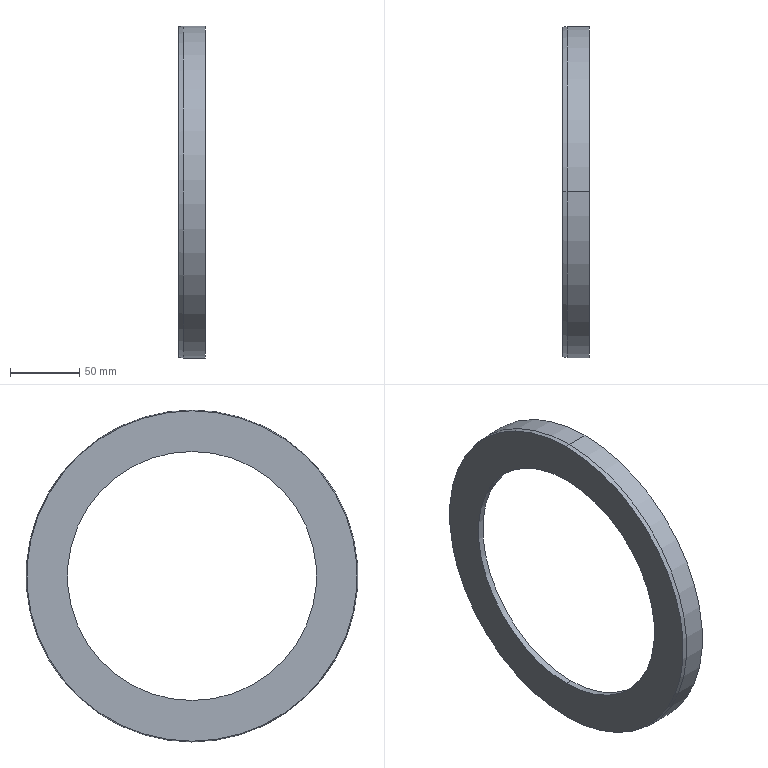Part | STEP file | Retaining ring | 1 solid | 13 faces | box 19 x 240 x 240 mm | volume 192307 mm3 | cylinder 6 | cone 4 | plane 3 | commonest cylinder face diameters 180 x2 220 x2 240 x2
STEP:
#1=CARTESIAN_POINT('',(0.,0.,0.));
#2=DIRECTION('',(0.,0.,1.));
#3=DIRECTION('',(1.,0.,0.));
#4=AXIS2_PLACEMENT_3D('',#1,#2,#3);
#5=CARTESIAN_POINT('',(4.5,0.,90.));
#6=VERTEX_POINT('',#5);
#7=CARTESIAN_POINT('',(0.,0.,90.));
#8=VERTEX_POINT('',#7);
#9=CARTESIAN_POINT('',(0.,0.,90.));
#10=DIRECTION('',(-1.,0.,0.));
#11=VECTOR('',#10,1.);
#12=LINE('',#9,#11);
#13=CARTESIAN_POINT('',(0.,0.,0.));
#14=DIRECTION('',(-1.,0.,0.));
#15=DIRECTION('',(0.,0.,1.));
#16=AXIS2_PLACEMENT_3D('',#13,#14,#15);
#17=CYLINDRICAL_SURFACE('',#16,90.);
#18=CARTESIAN_POINT('',(6.283,0.));
#19=DIRECTION('',(0.,1.));
#20=VECTOR('',#19,1.);
#21=LINE('',#18,#20);
#22=(GEOMETRIC_REPRESENTATION_CONTEXT(2)PARAMETRIC_REPRESENTATION_CONTEXT()REPRESENTATION_CONTEXT('',''));
#23=DEFINITIONAL_REPRESENTATION('',(#21),#22);
#24=PCURVE('',#17,#23);
#25=CARTESIAN_POINT('',(0.,0.,0.));
#26=DIRECTION('',(-1.,0.,0.));
#27=DIRECTION('',(0.,0.,1.));
#28=AXIS2_PLACEMENT_3D('',#25,#26,#27);
#29=CYLINDRICAL_SURFACE('',#28,90.);
#30=CARTESIAN_POINT('',(0.,0.));
#31=DIRECTION('',(0.,1.));
#32=VECTOR('',#31,1.);
#33=LINE('',#30,#32);
#34=(GEOMETRIC_REPRESENTATION_CONTEXT(2)PARAMETRIC_REPRESENTATION_CONTEXT()REPRESENTATION_CONTEXT('',''));
#35=DEFINITIONAL_REPRESENTATION('',(#33),#34);
#36=PCURVE('',#29,#35);
#37=SURFACE_CURVE('',#12,(#24,#36),.PCURVE_S1.);
#38=EDGE_CURVE('',#6,#8,#37,.T.);
#39=ORIENTED_EDGE('',*,*,#38,.T.);
#40=CARTESIAN_POINT('',(0.,0.,-90.));
#41=VERTEX_POINT('',#40);
#42=CARTESIAN_POINT('',(0.,0.,0.));
#43=DIRECTION('',(-1.,0.,0.));
#44=DIRECTION('',(0.,0.,1.));
#45=AXIS2_PLACEMENT_3D('',#42,#43,#44);
#46=CIRCLE('',#45,90.);
#47=CARTESIAN_POINT('',(0.,0.));
#48=DIRECTION('',(1.,0.));
#49=VECTOR('',#48,1.);
#50=LINE('',#47,#49);
#51=(GEOMETRIC_REPRESENTATION_CONTEXT(2)PARAMETRIC_REPRESENTATION_CONTEXT()REPRESENTATION_CONTEXT('',''));
#52=DEFINITIONAL_REPRESENTATION('',(#50),#51);
#53=PCURVE('',#17,#52);
#54=CARTESIAN_POINT('',(0.,-90.,0.));
#55=DIRECTION('',(-1.,0.,0.));
#56=DIRECTION('',(0.,0.,1.));
#57=AXIS2_PLACEMENT_3D('',#54,#55,#56);
#58=PLANE('',#57);
#59=CARTESIAN_POINT('',(0.,90.));
#60=DIRECTION('',(1.,0.));
#61=AXIS2_PLACEMENT_2D('',#59,#60);
#62=CIRCLE('',#61,90.);
#63=(GEOMETRIC_REPRESENTATION_CONTEXT(2)PARAMETRIC_REPRESENTATION_CONTEXT()REPRESENTATION_CONTEXT('',''));
#64=DEFINITIONAL_REPRESENTATION('',(#62),#63);
#65=PCURVE('',#58,#64);
#66=SURFACE_CURVE('',#46,(#53,#65),.PCURVE_S1.);
#67=EDGE_CURVE('',#41,#8,#66,.T.);
#68=ORIENTED_EDGE('',*,*,#67,.F.);
#69=CARTESIAN_POINT('',(4.5,0.,-90.));
#70=VERTEX_POINT('',#69);
#71=CARTESIAN_POINT('',(0.,0.,-90.));
#72=DIRECTION('',(-1.,0.,0.));
#73=VECTOR('',#72,1.);
#74=LINE('',#71,#73);
#75=CARTESIAN_POINT('',(3.142,0.));
#76=DIRECTION('',(0.,1.));
#77=VECTOR('',#76,1.);
#78=LINE('',#75,#77);
#79=(GEOMETRIC_REPRESENTATION_CONTEXT(2)PARAMETRIC_REPRESENTATION_CONTEXT()REPRESENTATION_CONTEXT('',''));
#80=DEFINITIONAL_REPRESENTATION('',(#78),#79);
#81=PCURVE('',#17,#80);
#82=CARTESIAN_POINT('',(3.142,0.));
#83=DIRECTION('',(0.,1.));
#84=VECTOR('',#83,1.);
#85=LINE('',#82,#84);
#86=(GEOMETRIC_REPRESENTATION_CONTEXT(2)PARAMETRIC_REPRESENTATION_CONTEXT()REPRESENTATION_CONTEXT('',''));
#87=DEFINITIONAL_REPRESENTATION('',(#85),#86);
#88=PCURVE('',#29,#87);
#89=SURFACE_CURVE('',#74,(#81,#88),.PCURVE_S1.);
#90=EDGE_CURVE('',#70,#41,#89,.T.);
#91=ORIENTED_EDGE('',*,*,#90,.F.);
#92=CARTESIAN_POINT('',(4.5,0.,0.));
#93=DIRECTION('',(-1.,0.,0.));
#94=DIRECTION('',(0.,0.,1.));
#95=AXIS2_PLACEMENT_3D('',#92,#93,#94);
#96=CIRCLE('',#95,90.);
#97=CARTESIAN_POINT('',(0.,-4.5));
#98=DIRECTION('',(1.,0.));
#99=VECTOR('',#98,1.);
#100=LINE('',#97,#99);
#101=(GEOMETRIC_REPRESENTATION_CONTEXT(2)PARAMETRIC_REPRESENTATION_CONTEXT()REPRESENTATION_CONTEXT('',''));
#102=DEFINITIONAL_REPRESENTATION('',(#100),#101);
#103=PCURVE('',#17,#102);
#104=CARTESIAN_POINT('',(4.5,-90.,0.));
#105=DIRECTION('',(1.,0.,0.));
#106=DIRECTION('',(0.,0.,-1.));
#107=AXIS2_PLACEMENT_3D('',#104,#105,#106);
#108=PLANE('',#107);
#109=CARTESIAN_POINT('',(-90.,90.));
#110=CARTESIAN_POINT('',(-90.,245.885));
#111=CARTESIAN_POINT('',(45.,167.942));
#112=CARTESIAN_POINT('',(180.,90.));
#113=CARTESIAN_POINT('',(45.,12.058));
#114=CARTESIAN_POINT('',(-90.,-65.885));
#115=CARTESIAN_POINT('',(-90.,90.));
#116=(BOUNDED_CURVE()B_SPLINE_CURVE(2,(#109,#110,#111,#112,#113,#114,#115),.UNSPECIFIED.,.T.,.F.)B_SPLINE_CURVE_WITH_KNOTS((1,2,2,2,2,1),(-2.094,0.,2.094,4.189,6.283,8.378),.UNSPECIFIED.)CURVE()GEOMETRIC_REPRESENTATION_ITEM()RATIONAL_B_SPLINE_CURVE((1.,0.5,1.,0.5,1.,0.5,1.))REPRESENTATION_ITEM(''));
#117=(GEOMETRIC_REPRESENTATION_CONTEXT(2)PARAMETRIC_REPRESENTATION_CONTEXT()REPRESENTATION_CONTEXT('',''));
#118=DEFINITIONAL_REPRESENTATION('',(#116),#117);
#119=PCURVE('',#108,#118);
#120=SURFACE_CURVE('',#96,(#103,#119),.PCURVE_S1.);
#121=EDGE_CURVE('',#70,#6,#120,.T.);
#122=ORIENTED_EDGE('',*,*,#121,.T.);
#123=EDGE_LOOP('',(#39,#68,#91,#122));
#124=FACE_BOUND('',#123,.F.);
#125=ADVANCED_FACE('',(#124),#17,.F.);
#126=CARTESIAN_POINT('',(0.,0.,119.408));
#127=VERTEX_POINT('',#126);
#128=CARTESIAN_POINT('',(0.,0.,-119.408));
#129=VERTEX_POINT('',#128);
#130=CARTESIAN_POINT('',(0.,0.,0.));
#131=DIRECTION('',(-1.,0.,0.));
#132=DIRECTION('',(0.,0.,1.));
#133=AXIS2_PLACEMENT_3D('',#130,#131,#132);
#134=CIRCLE('',#133,119.408);
#135=CARTESIAN_POINT('',(0.,0.,0.));
#136=DIRECTION('',(1.,0.,0.));
#137=DIRECTION('',(0.,0.,-1.));
#138=AXIS2_PLACEMENT_3D('',#135,#136,#137);
#139=CONICAL_SURFACE('',#138,119.408,0.1948);
#140=CARTESIAN_POINT('',(3.142,0.));
#141=DIRECTION('',(-1.,0.));
#142=VECTOR('',#141,1.);
#143=LINE('',#140,#142);
#144=(GEOMETRIC_REPRESENTATION_CONTEXT(2)PARAMETRIC_REPRESENTATION_CONTEXT()REPRESENTATION_CONTEXT('',''));
#145=DEFINITIONAL_REPRESENTATION('',(#143),#144);
#146=PCURVE('',#139,#145);
#147=CARTESIAN_POINT('',(0.,90.));
#148=DIRECTION('',(1.,0.));
#149=AXIS2_PLACEMENT_2D('',#147,#148);
#150=CIRCLE('',#149,119.408);
#151=(GEOMETRIC_REPRESENTATION_CONTEXT(2)PARAMETRIC_REPRESENTATION_CONTEXT()REPRESENTATION_CONTEXT('',''));
#152=DEFINITIONAL_REPRESENTATION('',(#150),#151);
#153=PCURVE('',#58,#152);
#154=SURFACE_CURVE('',#134,(#146,#153),.PCURVE_S1.);
#155=EDGE_CURVE('',#127,#129,#154,.T.);
#156=ORIENTED_EDGE('',*,*,#155,.F.);
#157=CARTESIAN_POINT('',(3.,0.,120.));
#158=VERTEX_POINT('',#157);
#159=CARTESIAN_POINT('',(0.,0.,119.408));
#160=DIRECTION('',(0.9811,0.,0.1936));
#161=VECTOR('',#160,1.);
#162=LINE('',#159,#161);
#163=CARTESIAN_POINT('',(3.142,0.));
#164=DIRECTION('',(0.,1.));
#165=VECTOR('',#164,1.);
#166=LINE('',#163,#165);
#167=(GEOMETRIC_REPRESENTATION_CONTEXT(2)PARAMETRIC_REPRESENTATION_CONTEXT()REPRESENTATION_CONTEXT('',''));
#168=DEFINITIONAL_REPRESENTATION('',(#166),#167);
#169=PCURVE('',#139,#168);
#170=CARTESIAN_POINT('',(0.,0.,0.));
#171=DIRECTION('',(1.,0.,0.));
#172=DIRECTION('',(0.,0.,-1.));
#173=AXIS2_PLACEMENT_3D('',#170,#171,#172);
#174=CONICAL_SURFACE('',#173,119.408,0.1948);
#175=CARTESIAN_POINT('',(3.142,0.));
#176=DIRECTION('',(0.,1.));
#177=VECTOR('',#176,1.);
#178=LINE('',#175,#177);
#179=(GEOMETRIC_REPRESENTATION_CONTEXT(2)PARAMETRIC_REPRESENTATION_CONTEXT()REPRESENTATION_CONTEXT('',''));
#180=DEFINITIONAL_REPRESENTATION('',(#178),#179);
#181=PCURVE('',#174,#180);
#182=SURFACE_CURVE('',#162,(#169,#181),.PCURVE_S1.);
#183=EDGE_CURVE('',#127,#158,#182,.T.);
#184=ORIENTED_EDGE('',*,*,#183,.T.);
#185=CARTESIAN_POINT('',(3.,0.,-120.));
#186=VERTEX_POINT('',#185);
#187=CARTESIAN_POINT('',(3.,0.,0.));
#188=DIRECTION('',(-1.,0.,0.));
#189=DIRECTION('',(0.,0.,1.));
#190=AXIS2_PLACEMENT_3D('',#187,#188,#189);
#191=CIRCLE('',#190,120.);
#192=CARTESIAN_POINT('',(3.142,3.));
#193=DIRECTION('',(-1.,0.));
#194=VECTOR('',#193,1.);
#195=LINE('',#192,#194);
#196=(GEOMETRIC_REPRESENTATION_CONTEXT(2)PARAMETRIC_REPRESENTATION_CONTEXT()REPRESENTATION_CONTEXT('',''));
#197=DEFINITIONAL_REPRESENTATION('',(#195),#196);
#198=PCURVE('',#139,#197);
#199=CARTESIAN_POINT('',(0.,0.,0.));
#200=DIRECTION('',(-1.,0.,0.));
#201=DIRECTION('',(0.,0.,1.));
#202=AXIS2_PLACEMENT_3D('',#199,#200,#201);
#203=CYLINDRICAL_SURFACE('',#202,120.);
#204=CARTESIAN_POINT('',(0.,-3.));
#205=DIRECTION('',(1.,0.));
#206=VECTOR('',#205,1.);
#207=LINE('',#204,#206);
#208=(GEOMETRIC_REPRESENTATION_CONTEXT(2)PARAMETRIC_REPRESENTATION_CONTEXT()REPRESENTATION_CONTEXT('',''));
#209=DEFINITIONAL_REPRESENTATION('',(#207),#208);
#210=PCURVE('',#203,#209);
#211=SURFACE_CURVE('',#191,(#198,#210),.PCURVE_S1.);
#212=EDGE_CURVE('',#158,#186,#211,.T.);
#213=ORIENTED_EDGE('',*,*,#212,.T.);
#214=CARTESIAN_POINT('',(0.,0.,-119.408));
#215=DIRECTION('',(0.9811,0.,-0.1936));
#216=VECTOR('',#215,1.);
#217=LINE('',#214,#216);
#218=CARTESIAN_POINT('',(0.,0.));
#219=DIRECTION('',(0.,1.));
#220=VECTOR('',#219,1.);
#221=LINE('',#218,#220);
#222=(GEOMETRIC_REPRESENTATION_CONTEXT(2)PARAMETRIC_REPRESENTATION_CONTEXT()REPRESENTATION_CONTEXT('',''));
#223=DEFINITIONAL_REPRESENTATION('',(#221),#222);
#224=PCURVE('',#139,#223);
#225=CARTESIAN_POINT('',(6.283,0.));
#226=DIRECTION('',(0.,1.));
#227=VECTOR('',#226,1.);
#228=LINE('',#225,#227);
#229=(GEOMETRIC_REPRESENTATION_CONTEXT(2)PARAMETRIC_REPRESENTATION_CONTEXT()REPRESENTATION_CONTEXT('',''));
#230=DEFINITIONAL_REPRESENTATION('',(#228),#229);
#231=PCURVE('',#174,#230);
#232=SURFACE_CURVE('',#217,(#224,#231),.PCURVE_S1.);
#233=EDGE_CURVE('',#129,#186,#232,.T.);
#234=ORIENTED_EDGE('',*,*,#233,.F.);
#235=EDGE_LOOP('',(#156,#184,#213,#234));
#236=FACE_BOUND('',#235,.T.);
#237=ADVANCED_FACE('',(#236),#139,.T.);
#238=CARTESIAN_POINT('',(19.,0.,120.));
#239=VERTEX_POINT('',#238);
#240=CARTESIAN_POINT('',(19.,0.,-120.));
#241=VERTEX_POINT('',#240);
#242=CARTESIAN_POINT('',(19.,0.,0.));
#243=DIRECTION('',(-1.,0.,0.));
#244=DIRECTION('',(0.,0.,1.));
#245=AXIS2_PLACEMENT_3D('',#242,#243,#244);
#246=CIRCLE('',#245,120.);
#247=CARTESIAN_POINT('',(0.,-19.));
#248=DIRECTION('',(1.,0.));
#249=VECTOR('',#248,1.);
#250=LINE('',#247,#249);
#251=(GEOMETRIC_REPRESENTATION_CONTEXT(2)PARAMETRIC_REPRESENTATION_CONTEXT()REPRESENTATION_CONTEXT('',''));
#252=DEFINITIONAL_REPRESENTATION('',(#250),#251);
#253=PCURVE('',#203,#252);
#254=CARTESIAN_POINT('',(19.,-112.473,0.));
#255=DIRECTION('',(1.,0.,0.));
#256=DIRECTION('',(0.,0.,-1.));
#257=AXIS2_PLACEMENT_3D('',#254,#255,#256);
#258=PLANE('',#257);
#259=CARTESIAN_POINT('',(-120.,112.473));
#260=CARTESIAN_POINT('',(-120.,320.32));
#261=CARTESIAN_POINT('',(60.,216.397));
#262=CARTESIAN_POINT('',(240.,112.473));
#263=CARTESIAN_POINT('',(60.,8.55));
#264=CARTESIAN_POINT('',(-120.,-95.373));
#265=CARTESIAN_POINT('',(-120.,112.473));
#266=(BOUNDED_CURVE()B_SPLINE_CURVE(2,(#259,#260,#261,#262,#263,#264,#265),.UNSPECIFIED.,.T.,.F.)B_SPLINE_CURVE_WITH_KNOTS((1,2,2,2,2,1),(-2.094,0.,2.094,4.189,6.283,8.378),.UNSPECIFIED.)CURVE()GEOMETRIC_REPRESENTATION_ITEM()RATIONAL_B_SPLINE_CURVE((1.,0.5,1.,0.5,1.,0.5,1.))REPRESENTATION_ITEM(''));
#267=(GEOMETRIC_REPRESENTATION_CONTEXT(2)PARAMETRIC_REPRESENTATION_CONTEXT()REPRESENTATION_CONTEXT('',''));
#268=DEFINITIONAL_REPRESENTATION('',(#266),#267);
#269=PCURVE('',#258,#268);
#270=SURFACE_CURVE('',#246,(#253,#269),.PCURVE_S1.);
#271=EDGE_CURVE('',#239,#241,#270,.T.);
#272=ORIENTED_EDGE('',*,*,#271,.T.);
#273=CARTESIAN_POINT('',(0.,0.,-120.));
#274=DIRECTION('',(-1.,0.,0.));
#275=VECTOR('',#274,1.);
#276=LINE('',#273,#275);
#277=CARTESIAN_POINT('',(3.142,0.));
#278=DIRECTION('',(0.,1.));
#279=VECTOR('',#278,1.);
#280=LINE('',#277,#279);
#281=(GEOMETRIC_REPRESENTATION_CONTEXT(2)PARAMETRIC_REPRESENTATION_CONTEXT()REPRESENTATION_CONTEXT('',''));
#282=DEFINITIONAL_REPRESENTATION('',(#280),#281);
#283=PCURVE('',#203,#282);
#284=CARTESIAN_POINT('',(0.,0.,0.));
#285=DIRECTION('',(-1.,0.,0.));
#286=DIRECTION('',(0.,0.,1.));
#287=AXIS2_PLACEMENT_3D('',#284,#285,#286);
#288=CYLINDRICAL_SURFACE('',#287,120.);
#289=CARTESIAN_POINT('',(3.142,0.));
#290=DIRECTION('',(0.,1.));
#291=VECTOR('',#290,1.);
#292=LINE('',#289,#291);
#293=(GEOMETRIC_REPRESENTATION_CONTEXT(2)PARAMETRIC_REPRESENTATION_CONTEXT()REPRESENTATION_CONTEXT('',''));
#294=DEFINITIONAL_REPRESENTATION('',(#292),#293);
#295=PCURVE('',#288,#294);
#296=SURFACE_CURVE('',#276,(#283,#295),.PCURVE_S1.);
#297=EDGE_CURVE('',#241,#186,#296,.T.);
#298=ORIENTED_EDGE('',*,*,#297,.T.);
#299=ORIENTED_EDGE('',*,*,#212,.F.);
#300=CARTESIAN_POINT('',(0.,0.,120.));
#301=DIRECTION('',(-1.,0.,0.));
#302=VECTOR('',#301,1.);
#303=LINE('',#300,#302);
#304=CARTESIAN_POINT('',(0.,0.));
#305=DIRECTION('',(0.,1.));
#306=VECTOR('',#305,1.);
#307=LINE('',#304,#306);
#308=(GEOMETRIC_REPRESENTATION_CONTEXT(2)PARAMETRIC_REPRESENTATION_CONTEXT()REPRESENTATION_CONTEXT('',''));
#309=DEFINITIONAL_REPRESENTATION('',(#307),#308);
#310=PCURVE('',#203,#309);
#311=CARTESIAN_POINT('',(6.283,0.));
#312=DIRECTION('',(0.,1.));
#313=VECTOR('',#312,1.);
#314=LINE('',#311,#313);
#315=(GEOMETRIC_REPRESENTATION_CONTEXT(2)PARAMETRIC_REPRESENTATION_CONTEXT()REPRESENTATION_CONTEXT('',''));
#316=DEFINITIONAL_REPRESENTATION('',(#314),#315);
#317=PCURVE('',#288,#316);
#318=SURFACE_CURVE('',#303,(#310,#317),.PCURVE_S1.);
#319=EDGE_CURVE('',#239,#158,#318,.T.);
#320=ORIENTED_EDGE('',*,*,#319,.F.);
#321=EDGE_LOOP('',(#272,#298,#299,#320));
#322=FACE_BOUND('',#321,.T.);
#323=ADVANCED_FACE('',(#322),#203,.T.);
#324=CARTESIAN_POINT('',(18.,0.,-110.));
#325=VERTEX_POINT('',#324);
#326=CARTESIAN_POINT('',(19.,0.,-112.473));
#327=VERTEX_POINT('',#326);
#328=CARTESIAN_POINT('',(19.,0.,-112.473));
#329=DIRECTION('',(0.3748,0.,-0.9271));
#330=VECTOR('',#329,1.);
#331=LINE('',#328,#330);
#332=CARTESIAN_POINT('',(19.,0.,0.));
#333=DIRECTION('',(1.,0.,0.));
#334=DIRECTION('',(0.,0.,-1.));
#335=AXIS2_PLACEMENT_3D('',#332,#333,#334);
#336=CONICAL_SURFACE('',#335,112.473,1.187);
#337=CARTESIAN_POINT('',(6.283,0.));
#338=DIRECTION('',(0.,1.));
#339=VECTOR('',#338,1.);
#340=LINE('',#337,#339);
#341=(GEOMETRIC_REPRESENTATION_CONTEXT(2)PARAMETRIC_REPRESENTATION_CONTEXT()REPRESENTATION_CONTEXT('',''));
#342=DEFINITIONAL_REPRESENTATION('',(#340),#341);
#343=PCURVE('',#336,#342);
#344=CARTESIAN_POINT('',(19.,0.,0.));
#345=DIRECTION('',(1.,0.,0.));
#346=DIRECTION('',(0.,0.,-1.));
#347=AXIS2_PLACEMENT_3D('',#344,#345,#346);
#348=CONICAL_SURFACE('',#347,112.473,1.187);
#349=CARTESIAN_POINT('',(0.,0.));
#350=DIRECTION('',(0.,1.));
#351=VECTOR('',#350,1.);
#352=LINE('',#349,#351);
#353=(GEOMETRIC_REPRESENTATION_CONTEXT(2)PARAMETRIC_REPRESENTATION_CONTEXT()REPRESENTATION_CONTEXT('',''));
#354=DEFINITIONAL_REPRESENTATION('',(#352),#353);
#355=PCURVE('',#348,#354);
#356=SURFACE_CURVE('',#331,(#343,#355),.PCURVE_S1.);
#357=EDGE_CURVE('',#325,#327,#356,.T.);
#358=ORIENTED_EDGE('',*,*,#357,.T.);
#359=CARTESIAN_POINT('',(19.,0.,112.473));
#360=VERTEX_POINT('',#359);
#361=CARTESIAN_POINT('',(19.,0.,0.));
#362=DIRECTION('',(-1.,0.,0.));
#363=DIRECTION('',(0.,0.,1.));
#364=AXIS2_PLACEMENT_3D('',#361,#362,#363);
#365=CIRCLE('',#364,112.473);
#366=CARTESIAN_POINT('',(9.425,0.));
#367=DIRECTION('',(-1.,0.));
#368=VECTOR('',#367,1.);
#369=LINE('',#366,#368);
#370=(GEOMETRIC_REPRESENTATION_CONTEXT(2)PARAMETRIC_REPRESENTATION_CONTEXT()REPRESENTATION_CONTEXT('',''));
#371=DEFINITIONAL_REPRESENTATION('',(#369),#370);
#372=PCURVE('',#336,#371);
#373=CARTESIAN_POINT('',(-112.473,112.473));
#374=CARTESIAN_POINT('',(-112.473,307.283));
#375=CARTESIAN_POINT('',(56.237,209.878));
#376=CARTESIAN_POINT('',(224.947,112.473));
#377=CARTESIAN_POINT('',(56.237,15.069));
#378=CARTESIAN_POINT('',(-112.473,-82.336));
#379=CARTESIAN_POINT('',(-112.473,112.473));
#380=(BOUNDED_CURVE()B_SPLINE_CURVE(2,(#373,#374,#375,#376,#377,#378,#379),.UNSPECIFIED.,.T.,.F.)B_SPLINE_CURVE_WITH_KNOTS((1,2,2,2,2,1),(-2.094,0.,2.094,4.189,6.283,8.378),.UNSPECIFIED.)CURVE()GEOMETRIC_REPRESENTATION_ITEM()RATIONAL_B_SPLINE_CURVE((1.,0.5,1.,0.5,1.,0.5,1.))REPRESENTATION_ITEM(''));
#381=(GEOMETRIC_REPRESENTATION_CONTEXT(2)PARAMETRIC_REPRESENTATION_CONTEXT()REPRESENTATION_CONTEXT('',''));
#382=DEFINITIONAL_REPRESENTATION('',(#380),#381);
#383=PCURVE('',#258,#382);
#384=SURFACE_CURVE('',#365,(#372,#383),.PCURVE_S1.);
#385=EDGE_CURVE('',#327,#360,#384,.T.);
#386=ORIENTED_EDGE('',*,*,#385,.T.);
#387=CARTESIAN_POINT('',(18.,0.,110.));
#388=VERTEX_POINT('',#387);
#389=CARTESIAN_POINT('',(19.,0.,112.473));
#390=DIRECTION('',(0.3748,0.,0.9271));
#391=VECTOR('',#390,1.);
#392=LINE('',#389,#391);
#393=CARTESIAN_POINT('',(3.142,0.));
#394=DIRECTION('',(0.,1.));
#395=VECTOR('',#394,1.);
#396=LINE('',#393,#395);
#397=(GEOMETRIC_REPRESENTATION_CONTEXT(2)PARAMETRIC_REPRESENTATION_CONTEXT()REPRESENTATION_CONTEXT('',''));
#398=DEFINITIONAL_REPRESENTATION('',(#396),#397);
#399=PCURVE('',#336,#398);
#400=CARTESIAN_POINT('',(3.142,0.));
#401=DIRECTION('',(0.,1.));
#402=VECTOR('',#401,1.);
#403=LINE('',#400,#402);
#404=(GEOMETRIC_REPRESENTATION_CONTEXT(2)PARAMETRIC_REPRESENTATION_CONTEXT()REPRESENTATION_CONTEXT('',''));
#405=DEFINITIONAL_REPRESENTATION('',(#403),#404);
#406=PCURVE('',#348,#405);
#407=SURFACE_CURVE('',#392,(#399,#406),.PCURVE_S1.);
#408=EDGE_CURVE('',#388,#360,#407,.T.);
#409=ORIENTED_EDGE('',*,*,#408,.F.);
#410=CARTESIAN_POINT('',(18.,0.,0.));
#411=DIRECTION('',(-1.,0.,0.));
#412=DIRECTION('',(0.,0.,1.));
#413=AXIS2_PLACEMENT_3D('',#410,#411,#412);
#414=CIRCLE('',#413,110.);
#415=CARTESIAN_POINT('',(9.425,-1.));
#416=DIRECTION('',(-1.,0.));
#417=VECTOR('',#416,1.);
#418=LINE('',#415,#417);
#419=(GEOMETRIC_REPRESENTATION_CONTEXT(2)PARAMETRIC_REPRESENTATION_CONTEXT()REPRESENTATION_CONTEXT('',''));
#420=DEFINITIONAL_REPRESENTATION('',(#418),#419);
#421=PCURVE('',#336,#420);
#422=CARTESIAN_POINT('',(0.,0.,0.));
#423=DIRECTION('',(-1.,0.,0.));
#424=DIRECTION('',(0.,0.,1.));
#425=AXIS2_PLACEMENT_3D('',#422,#423,#424);
#426=CYLINDRICAL_SURFACE('',#425,110.);
#427=CARTESIAN_POINT('',(0.,-18.));
#428=DIRECTION('',(1.,0.));
#429=VECTOR('',#428,1.);
#430=LINE('',#427,#429);
#431=(GEOMETRIC_REPRESENTATION_CONTEXT(2)PARAMETRIC_REPRESENTATION_CONTEXT()REPRESENTATION_CONTEXT('',''));
#432=DEFINITIONAL_REPRESENTATION('',(#430),#431);
#433=PCURVE('',#426,#432);
#434=SURFACE_CURVE('',#414,(#421,#433),.PCURVE_S1.);
#435=EDGE_CURVE('',#325,#388,#434,.T.);
#436=ORIENTED_EDGE('',*,*,#435,.F.);
#437=EDGE_LOOP('',(#358,#386,#409,#436));
#438=FACE_BOUND('',#437,.F.);
#439=ADVANCED_FACE('',(#438),#336,.F.);
#440=CARTESIAN_POINT('',(4.5,0.,110.));
#441=VERTEX_POINT('',#440);
#442=CARTESIAN_POINT('',(0.,0.,110.));
#443=DIRECTION('',(-1.,0.,0.));
#444=VECTOR('',#443,1.);
#445=LINE('',#442,#444);
#446=CARTESIAN_POINT('',(6.283,0.));
#447=DIRECTION('',(0.,1.));
#448=VECTOR('',#447,1.);
#449=LINE('',#446,#448);
#450=(GEOMETRIC_REPRESENTATION_CONTEXT(2)PARAMETRIC_REPRESENTATION_CONTEXT()REPRESENTATION_CONTEXT('',''));
#451=DEFINITIONAL_REPRESENTATION('',(#449),#450);
#452=PCURVE('',#426,#451);
#453=CARTESIAN_POINT('',(0.,0.,0.));
#454=DIRECTION('',(-1.,0.,0.));
#455=DIRECTION('',(0.,0.,1.));
#456=AXIS2_PLACEMENT_3D('',#453,#454,#455);
#457=CYLINDRICAL_SURFACE('',#456,110.);
#458=CARTESIAN_POINT('',(0.,0.));
#459=DIRECTION('',(0.,1.));
#460=VECTOR('',#459,1.);
#461=LINE('',#458,#460);
#462=(GEOMETRIC_REPRESENTATION_CONTEXT(2)PARAMETRIC_REPRESENTATION_CONTEXT()REPRESENTATION_CONTEXT('',''));
#463=DEFINITIONAL_REPRESENTATION('',(#461),#462);
#464=PCURVE('',#457,#463);
#465=SURFACE_CURVE('',#445,(#452,#464),.PCURVE_S1.);
#466=EDGE_CURVE('',#388,#441,#465,.T.);
#467=ORIENTED_EDGE('',*,*,#466,.T.);
#468=CARTESIAN_POINT('',(4.5,0.,-110.));
#469=VERTEX_POINT('',#468);
#470=CARTESIAN_POINT('',(4.5,0.,0.));
#471=DIRECTION('',(-1.,0.,0.));
#472=DIRECTION('',(0.,0.,1.));
#473=AXIS2_PLACEMENT_3D('',#470,#471,#472);
#474=CIRCLE('',#473,110.);
#475=CARTESIAN_POINT('',(0.,-4.5));
#476=DIRECTION('',(1.,0.));
#477=VECTOR('',#476,1.);
#478=LINE('',#475,#477);
#479=(GEOMETRIC_REPRESENTATION_CONTEXT(2)PARAMETRIC_REPRESENTATION_CONTEXT()REPRESENTATION_CONTEXT('',''));
#480=DEFINITIONAL_REPRESENTATION('',(#478),#479);
#481=PCURVE('',#426,#480);
#482=CARTESIAN_POINT('',(-110.,90.));
#483=CARTESIAN_POINT('',(-110.,280.526));
#484=CARTESIAN_POINT('',(55.,185.263));
#485=CARTESIAN_POINT('',(220.,90.));
#486=CARTESIAN_POINT('',(55.,-5.263));
#487=CARTESIAN_POINT('',(-110.,-100.526));
#488=CARTESIAN_POINT('',(-110.,90.));
#489=(BOUNDED_CURVE()B_SPLINE_CURVE(2,(#482,#483,#484,#485,#486,#487,#488),.UNSPECIFIED.,.T.,.F.)B_SPLINE_CURVE_WITH_KNOTS((1,2,2,2,2,1),(-2.094,0.,2.094,4.189,6.283,8.378),.UNSPECIFIED.)CURVE()GEOMETRIC_REPRESENTATION_ITEM()RATIONAL_B_SPLINE_CURVE((1.,0.5,1.,0.5,1.,0.5,1.))REPRESENTATION_ITEM(''));
#490=(GEOMETRIC_REPRESENTATION_CONTEXT(2)PARAMETRIC_REPRESENTATION_CONTEXT()REPRESENTATION_CONTEXT('',''));
#491=DEFINITIONAL_REPRESENTATION('',(#489),#490);
#492=PCURVE('',#108,#491);
#493=SURFACE_CURVE('',#474,(#481,#492),.PCURVE_S1.);
#494=EDGE_CURVE('',#469,#441,#493,.T.);
#495=ORIENTED_EDGE('',*,*,#494,.F.);
#496=CARTESIAN_POINT('',(0.,0.,-110.));
#497=DIRECTION('',(-1.,0.,0.));
#498=VECTOR('',#497,1.);
#499=LINE('',#496,#498);
#500=CARTESIAN_POINT('',(3.142,0.));
#501=DIRECTION('',(0.,1.));
#502=VECTOR('',#501,1.);
#503=LINE('',#500,#502);
#504=(GEOMETRIC_REPRESENTATION_CONTEXT(2)PARAMETRIC_REPRESENTATION_CONTEXT()REPRESENTATION_CONTEXT('',''));
#505=DEFINITIONAL_REPRESENTATION('',(#503),#504);
#506=PCURVE('',#426,#505);
#507=CARTESIAN_POINT('',(3.142,0.));
#508=DIRECTION('',(0.,1.));
#509=VECTOR('',#508,1.);
#510=LINE('',#507,#509);
#511=(GEOMETRIC_REPRESENTATION_CONTEXT(2)PARAMETRIC_REPRESENTATION_CONTEXT()REPRESENTATION_CONTEXT('',''));
#512=DEFINITIONAL_REPRESENTATION('',(#510),#511);
#513=PCURVE('',#457,#512);
#514=SURFACE_CURVE('',#499,(#506,#513),.PCURVE_S1.);
#515=EDGE_CURVE('',#325,#469,#514,.T.);
#516=ORIENTED_EDGE('',*,*,#515,.F.);
#517=ORIENTED_EDGE('',*,*,#435,.T.);
#518=EDGE_LOOP('',(#467,#495,#516,#517));
#519=FACE_BOUND('',#518,.F.);
#520=ADVANCED_FACE('',(#519),#426,.F.);
#521=CARTESIAN_POINT('',(4.5,0.,0.));
#522=DIRECTION('',(-1.,0.,0.));
#523=DIRECTION('',(0.,0.,1.));
#524=AXIS2_PLACEMENT_3D('',#521,#522,#523);
#525=CIRCLE('',#524,110.);
#526=CARTESIAN_POINT('',(0.,-4.5));
#527=DIRECTION('',(1.,0.));
#528=VECTOR('',#527,1.);
#529=LINE('',#526,#528);
#530=(GEOMETRIC_REPRESENTATION_CONTEXT(2)PARAMETRIC_REPRESENTATION_CONTEXT()REPRESENTATION_CONTEXT('',''));
#531=DEFINITIONAL_REPRESENTATION('',(#529),#530);
#532=PCURVE('',#457,#531);
#533=CARTESIAN_POINT('',(-110.,90.));
#534=CARTESIAN_POINT('',(-110.,280.526));
#535=CARTESIAN_POINT('',(55.,185.263));
#536=CARTESIAN_POINT('',(220.,90.));
#537=CARTESIAN_POINT('',(55.,-5.263));
#538=CARTESIAN_POINT('',(-110.,-100.526));
#539=CARTESIAN_POINT('',(-110.,90.));
#540=(BOUNDED_CURVE()B_SPLINE_CURVE(2,(#533,#534,#535,#536,#537,#538,#539),.UNSPECIFIED.,.T.,.F.)B_SPLINE_CURVE_WITH_KNOTS((1,2,2,2,2,1),(-2.094,0.,2.094,4.189,6.283,8.378),.UNSPECIFIED.)CURVE()GEOMETRIC_REPRESENTATION_ITEM()RATIONAL_B_SPLINE_CURVE((1.,0.5,1.,0.5,1.,0.5,1.))REPRESENTATION_ITEM(''));
#541=(GEOMETRIC_REPRESENTATION_CONTEXT(2)PARAMETRIC_REPRESENTATION_CONTEXT()REPRESENTATION_CONTEXT('',''));
#542=DEFINITIONAL_REPRESENTATION('',(#540),#541);
#543=PCURVE('',#108,#542);
#544=SURFACE_CURVE('',#525,(#532,#543),.PCURVE_S1.);
#545=EDGE_CURVE('',#441,#469,#544,.T.);
#546=ORIENTED_EDGE('',*,*,#545,.F.);
#547=ORIENTED_EDGE('',*,*,#466,.F.);
#548=CARTESIAN_POINT('',(18.,0.,0.));
#549=DIRECTION('',(-1.,0.,0.));
#550=DIRECTION('',(0.,0.,1.));
#551=AXIS2_PLACEMENT_3D('',#548,#549,#550);
#552=CIRCLE('',#551,110.);
#553=CARTESIAN_POINT('',(0.,-18.));
#554=DIRECTION('',(1.,0.));
#555=VECTOR('',#554,1.);
#556=LINE('',#553,#555);
#557=(GEOMETRIC_REPRESENTATION_CONTEXT(2)PARAMETRIC_REPRESENTATION_CONTEXT()REPRESENTATION_CONTEXT('',''));
#558=DEFINITIONAL_REPRESENTATION('',(#556),#557);
#559=PCURVE('',#457,#558);
#560=CARTESIAN_POINT('',(3.142,-1.));
#561=DIRECTION('',(-1.,0.));
#562=VECTOR('',#561,1.);
#563=LINE('',#560,#562);
#564=(GEOMETRIC_REPRESENTATION_CONTEXT(2)PARAMETRIC_REPRESENTATION_CONTEXT()REPRESENTATION_CONTEXT('',''));
#565=DEFINITIONAL_REPRESENTATION('',(#563),#564);
#566=PCURVE('',#348,#565);
#567=SURFACE_CURVE('',#552,(#559,#566),.PCURVE_S1.);
#568=EDGE_CURVE('',#388,#325,#567,.T.);
#569=ORIENTED_EDGE('',*,*,#568,.T.);
#570=ORIENTED_EDGE('',*,*,#515,.T.);
#571=EDGE_LOOP('',(#546,#547,#569,#570));
#572=FACE_BOUND('',#571,.F.);
#573=ADVANCED_FACE('',(#572),#457,.F.);
#574=CARTESIAN_POINT('',(19.,0.,0.));
#575=DIRECTION('',(-1.,0.,0.));
#576=DIRECTION('',(0.,0.,1.));
#577=AXIS2_PLACEMENT_3D('',#574,#575,#576);
#578=CIRCLE('',#577,112.473);
#579=CARTESIAN_POINT('',(3.142,0.));
#580=DIRECTION('',(-1.,0.));
#581=VECTOR('',#580,1.);
#582=LINE('',#579,#581);
#583=(GEOMETRIC_REPRESENTATION_CONTEXT(2)PARAMETRIC_REPRESENTATION_CONTEXT()REPRESENTATION_CONTEXT('',''));
#584=DEFINITIONAL_REPRESENTATION('',(#582),#583);
#585=PCURVE('',#348,#584);
#586=CARTESIAN_POINT('',(-112.473,112.473));
#587=CARTESIAN_POINT('',(-112.473,307.283));
#588=CARTESIAN_POINT('',(56.237,209.878));
#589=CARTESIAN_POINT('',(224.947,112.473));
#590=CARTESIAN_POINT('',(56.237,15.069));
#591=CARTESIAN_POINT('',(-112.473,-82.336));
#592=CARTESIAN_POINT('',(-112.473,112.473));
#593=(BOUNDED_CURVE()B_SPLINE_CURVE(2,(#586,#587,#588,#589,#590,#591,#592),.UNSPECIFIED.,.T.,.F.)B_SPLINE_CURVE_WITH_KNOTS((1,2,2,2,2,1),(-2.094,0.,2.094,4.189,6.283,8.378),.UNSPECIFIED.)CURVE()GEOMETRIC_REPRESENTATION_ITEM()RATIONAL_B_SPLINE_CURVE((1.,0.5,1.,0.5,1.,0.5,1.))REPRESENTATION_ITEM(''));
#594=(GEOMETRIC_REPRESENTATION_CONTEXT(2)PARAMETRIC_REPRESENTATION_CONTEXT()REPRESENTATION_CONTEXT('',''));
#595=DEFINITIONAL_REPRESENTATION('',(#593),#594);
#596=PCURVE('',#258,#595);
#597=SURFACE_CURVE('',#578,(#585,#596),.PCURVE_S1.);
#598=EDGE_CURVE('',#360,#327,#597,.T.);
#599=ORIENTED_EDGE('',*,*,#598,.T.);
#600=ORIENTED_EDGE('',*,*,#357,.F.);
#601=ORIENTED_EDGE('',*,*,#568,.F.);
#602=ORIENTED_EDGE('',*,*,#408,.T.);
#603=EDGE_LOOP('',(#599,#600,#601,#602));
#604=FACE_BOUND('',#603,.F.);
#605=ADVANCED_FACE('',(#604),#348,.F.);
#606=ORIENTED_EDGE('',*,*,#385,.T.);
#607=ORIENTED_EDGE('',*,*,#598,.T.);
#608=EDGE_LOOP('',(#606,#607));
#609=FACE_BOUND('',#608,.T.);
#610=ORIENTED_EDGE('',*,*,#271,.F.);
#611=CARTESIAN_POINT('',(19.,0.,0.));
#612=DIRECTION('',(-1.,0.,0.));
#613=DIRECTION('',(0.,0.,1.));
#614=AXIS2_PLACEMENT_3D('',#611,#612,#613);
#615=CIRCLE('',#614,120.);
#616=CARTESIAN_POINT('',(-120.,112.473));
#617=CARTESIAN_POINT('',(-120.,320.32));
#618=CARTESIAN_POINT('',(60.,216.397));
#619=CARTESIAN_POINT('',(240.,112.473));
#620=CARTESIAN_POINT('',(60.,8.55));
#621=CARTESIAN_POINT('',(-120.,-95.373));
#622=CARTESIAN_POINT('',(-120.,112.473));
#623=(BOUNDED_CURVE()B_SPLINE_CURVE(2,(#616,#617,#618,#619,#620,#621,#622),.UNSPECIFIED.,.T.,.F.)B_SPLINE_CURVE_WITH_KNOTS((1,2,2,2,2,1),(-2.094,0.,2.094,4.189,6.283,8.378),.UNSPECIFIED.)CURVE()GEOMETRIC_REPRESENTATION_ITEM()RATIONAL_B_SPLINE_CURVE((1.,0.5,1.,0.5,1.,0.5,1.))REPRESENTATION_ITEM(''));
#624=(GEOMETRIC_REPRESENTATION_CONTEXT(2)PARAMETRIC_REPRESENTATION_CONTEXT()REPRESENTATION_CONTEXT('',''));
#625=DEFINITIONAL_REPRESENTATION('',(#623),#624);
#626=PCURVE('',#258,#625);
#627=CARTESIAN_POINT('',(0.,-19.));
#628=DIRECTION('',(1.,0.));
#629=VECTOR('',#628,1.);
#630=LINE('',#627,#629);
#631=(GEOMETRIC_REPRESENTATION_CONTEXT(2)PARAMETRIC_REPRESENTATION_CONTEXT()REPRESENTATION_CONTEXT('',''));
#632=DEFINITIONAL_REPRESENTATION('',(#630),#631);
#633=PCURVE('',#288,#632);
#634=SURFACE_CURVE('',#615,(#626,#633),.PCURVE_S1.);
#635=EDGE_CURVE('',#241,#239,#634,.T.);
#636=ORIENTED_EDGE('',*,*,#635,.F.);
#637=EDGE_LOOP('',(#610,#636));
#638=FACE_BOUND('',#637,.T.);
#639=ADVANCED_FACE('',(#609,#638),#258,.T.);
#640=ORIENTED_EDGE('',*,*,#297,.F.);
#641=ORIENTED_EDGE('',*,*,#635,.T.);
#642=ORIENTED_EDGE('',*,*,#319,.T.);
#643=CARTESIAN_POINT('',(3.,0.,0.));
#644=DIRECTION('',(-1.,0.,0.));
#645=DIRECTION('',(0.,0.,1.));
#646=AXIS2_PLACEMENT_3D('',#643,#644,#645);
#647=CIRCLE('',#646,120.);
#648=CARTESIAN_POINT('',(0.,-3.));
#649=DIRECTION('',(1.,0.));
#650=VECTOR('',#649,1.);
#651=LINE('',#648,#650);
#652=(GEOMETRIC_REPRESENTATION_CONTEXT(2)PARAMETRIC_REPRESENTATION_CONTEXT()REPRESENTATION_CONTEXT('',''));
#653=DEFINITIONAL_REPRESENTATION('',(#651),#652);
#654=PCURVE('',#288,#653);
#655=CARTESIAN_POINT('',(9.425,3.));
#656=DIRECTION('',(-1.,0.));
#657=VECTOR('',#656,1.);
#658=LINE('',#655,#657);
#659=(GEOMETRIC_REPRESENTATION_CONTEXT(2)PARAMETRIC_REPRESENTATION_CONTEXT()REPRESENTATION_CONTEXT('',''));
#660=DEFINITIONAL_REPRESENTATION('',(#658),#659);
#661=PCURVE('',#174,#660);
#662=SURFACE_CURVE('',#647,(#654,#661),.PCURVE_S1.);
#663=EDGE_CURVE('',#186,#158,#662,.T.);
#664=ORIENTED_EDGE('',*,*,#663,.F.);
#665=EDGE_LOOP('',(#640,#641,#642,#664));
#666=FACE_BOUND('',#665,.T.);
#667=ADVANCED_FACE('',(#666),#288,.T.);
#668=ORIENTED_EDGE('',*,*,#183,.F.);
#669=CARTESIAN_POINT('',(0.,0.,0.));
#670=DIRECTION('',(-1.,0.,0.));
#671=DIRECTION('',(0.,0.,1.));
#672=AXIS2_PLACEMENT_3D('',#669,#670,#671);
#673=CIRCLE('',#672,119.408);
#674=CARTESIAN_POINT('',(9.425,0.));
#675=DIRECTION('',(-1.,0.));
#676=VECTOR('',#675,1.);
#677=LINE('',#674,#676);
#678=(GEOMETRIC_REPRESENTATION_CONTEXT(2)PARAMETRIC_REPRESENTATION_CONTEXT()REPRESENTATION_CONTEXT('',''));
#679=DEFINITIONAL_REPRESENTATION('',(#677),#678);
#680=PCURVE('',#174,#679);
#681=CARTESIAN_POINT('',(0.,90.));
#682=DIRECTION('',(1.,0.));
#683=AXIS2_PLACEMENT_2D('',#681,#682);
#684=CIRCLE('',#683,119.408);
#685=(GEOMETRIC_REPRESENTATION_CONTEXT(2)PARAMETRIC_REPRESENTATION_CONTEXT()REPRESENTATION_CONTEXT('',''));
#686=DEFINITIONAL_REPRESENTATION('',(#684),#685);
#687=PCURVE('',#58,#686);
#688=SURFACE_CURVE('',#673,(#680,#687),.PCURVE_S1.);
#689=EDGE_CURVE('',#129,#127,#688,.T.);
#690=ORIENTED_EDGE('',*,*,#689,.F.);
#691=ORIENTED_EDGE('',*,*,#233,.T.);
#692=ORIENTED_EDGE('',*,*,#663,.T.);
#693=EDGE_LOOP('',(#668,#690,#691,#692));
#694=FACE_BOUND('',#693,.T.);
#695=ADVANCED_FACE('',(#694),#174,.T.);
#696=ORIENTED_EDGE('',*,*,#689,.T.);
#697=ORIENTED_EDGE('',*,*,#155,.T.);
#698=EDGE_LOOP('',(#696,#697));
#699=FACE_BOUND('',#698,.T.);
#700=CARTESIAN_POINT('',(0.,0.,0.));
#701=DIRECTION('',(-1.,0.,0.));
#702=DIRECTION('',(0.,0.,1.));
#703=AXIS2_PLACEMENT_3D('',#700,#701,#702);
#704=CIRCLE('',#703,90.);
#705=CARTESIAN_POINT('',(0.,90.));
#706=DIRECTION('',(1.,0.));
#707=AXIS2_PLACEMENT_2D('',#705,#706);
#708=CIRCLE('',#707,90.);
#709=(GEOMETRIC_REPRESENTATION_CONTEXT(2)PARAMETRIC_REPRESENTATION_CONTEXT()REPRESENTATION_CONTEXT('',''));
#710=DEFINITIONAL_REPRESENTATION('',(#708),#709);
#711=PCURVE('',#58,#710);
#712=CARTESIAN_POINT('',(0.,0.));
#713=DIRECTION('',(1.,0.));
#714=VECTOR('',#713,1.);
#715=LINE('',#712,#714);
#716=(GEOMETRIC_REPRESENTATION_CONTEXT(2)PARAMETRIC_REPRESENTATION_CONTEXT()REPRESENTATION_CONTEXT('',''));
#717=DEFINITIONAL_REPRESENTATION('',(#715),#716);
#718=PCURVE('',#29,#717);
#719=SURFACE_CURVE('',#704,(#711,#718),.PCURVE_S1.);
#720=EDGE_CURVE('',#8,#41,#719,.T.);
#721=ORIENTED_EDGE('',*,*,#720,.F.);
#722=ORIENTED_EDGE('',*,*,#67,.F.);
#723=EDGE_LOOP('',(#721,#722));
#724=FACE_BOUND('',#723,.T.);
#725=ADVANCED_FACE('',(#699,#724),#58,.T.);
#726=ORIENTED_EDGE('',*,*,#720,.F.);
#727=ORIENTED_EDGE('',*,*,#38,.F.);
#728=CARTESIAN_POINT('',(4.5,0.,0.));
#729=DIRECTION('',(-1.,0.,0.));
#730=DIRECTION('',(0.,0.,1.));
#731=AXIS2_PLACEMENT_3D('',#728,#729,#730);
#732=CIRCLE('',#731,90.);
#733=CARTESIAN_POINT('',(0.,-4.5));
#734=DIRECTION('',(1.,0.));
#735=VECTOR('',#734,1.);
#736=LINE('',#733,#735);
#737=(GEOMETRIC_REPRESENTATION_CONTEXT(2)PARAMETRIC_REPRESENTATION_CONTEXT()REPRESENTATION_CONTEXT('',''));
#738=DEFINITIONAL_REPRESENTATION('',(#736),#737);
#739=PCURVE('',#29,#738);
#740=CARTESIAN_POINT('',(-90.,90.));
#741=CARTESIAN_POINT('',(-90.,245.885));
#742=CARTESIAN_POINT('',(45.,167.942));
#743=CARTESIAN_POINT('',(180.,90.));
#744=CARTESIAN_POINT('',(45.,12.058));
#745=CARTESIAN_POINT('',(-90.,-65.885));
#746=CARTESIAN_POINT('',(-90.,90.));
#747=(BOUNDED_CURVE()B_SPLINE_CURVE(2,(#740,#741,#742,#743,#744,#745,#746),.UNSPECIFIED.,.T.,.F.)B_SPLINE_CURVE_WITH_KNOTS((1,2,2,2,2,1),(-2.094,0.,2.094,4.189,6.283,8.378),.UNSPECIFIED.)CURVE()GEOMETRIC_REPRESENTATION_ITEM()RATIONAL_B_SPLINE_CURVE((1.,0.5,1.,0.5,1.,0.5,1.))REPRESENTATION_ITEM(''));
#748=(GEOMETRIC_REPRESENTATION_CONTEXT(2)PARAMETRIC_REPRESENTATION_CONTEXT()REPRESENTATION_CONTEXT('',''));
#749=DEFINITIONAL_REPRESENTATION('',(#747),#748);
#750=PCURVE('',#108,#749);
#751=SURFACE_CURVE('',#732,(#739,#750),.PCURVE_S1.);
#752=EDGE_CURVE('',#6,#70,#751,.T.);
#753=ORIENTED_EDGE('',*,*,#752,.T.);
#754=ORIENTED_EDGE('',*,*,#90,.T.);
#755=EDGE_LOOP('',(#726,#727,#753,#754));
#756=FACE_BOUND('',#755,.F.);
#757=ADVANCED_FACE('',(#756),#29,.F.);
#758=ORIENTED_EDGE('',*,*,#752,.T.);
#759=ORIENTED_EDGE('',*,*,#121,.T.);
#760=EDGE_LOOP('',(#758,#759));
#761=FACE_BOUND('',#760,.T.);
#762=ORIENTED_EDGE('',*,*,#545,.F.);
#763=ORIENTED_EDGE('',*,*,#494,.F.);
#764=EDGE_LOOP('',(#762,#763));
#765=FACE_BOUND('',#764,.T.);
#766=ADVANCED_FACE('',(#761,#765),#108,.T.);
#767=CLOSED_SHELL('',(#125,#237,#323,#439,#520,#573,#605,#639,#667,#695,#725,#757,#766));
#768=MANIFOLD_SOLID_BREP('',#767);
#769=(LENGTH_UNIT()NAMED_UNIT(*)SI_UNIT(.MILLI.,.METRE.));
#770=UNCERTAINTY_MEASURE_WITH_UNIT(LENGTH_MEASURE(0.0000001),#769,'','');
#771=(NAMED_UNIT(*)PLANE_ANGLE_UNIT()SI_UNIT($,.RADIAN.));
#772=(NAMED_UNIT(*)SI_UNIT($,.STERADIAN.)SOLID_ANGLE_UNIT());
#773=(GEOMETRIC_REPRESENTATION_CONTEXT(3)GLOBAL_UNCERTAINTY_ASSIGNED_CONTEXT((#770))GLOBAL_UNIT_ASSIGNED_CONTEXT((#769,#771,#772))REPRESENTATION_CONTEXT('',''));
#774=ADVANCED_BREP_SHAPE_REPRESENTATION('',(#4,#768),#773);